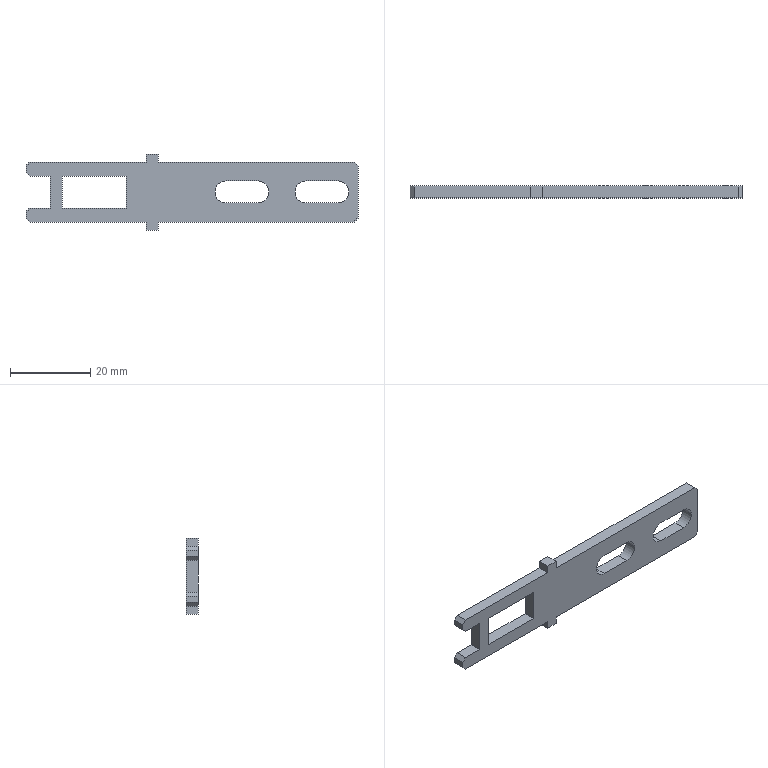Part | NX | features solid 2 | 1 solid | 38 faces | box 83 x 3 x 19 mm | volume 2827 mm3 | plane 32 | cylinder 6 | commonest cylinder face diameters 5.5 x6
STEP:
#1=CARTESIAN_POINT('',(-284.034,-1543.5,1313.749));
#2=VERTEX_POINT('',#1);
#3=CARTESIAN_POINT('',(-284.034,-1540.5,1313.749));
#4=VERTEX_POINT('',#3);
#5=CARTESIAN_POINT('',(-284.034,-1625.7,1313.749));
#6=DIRECTION('',(0.,1.,0.));
#7=VECTOR('',#6,1000.);
#8=LINE('',#5,#7);
#9=EDGE_CURVE('',#2,#4,#8,.T.);
#10=ORIENTED_EDGE('',*,*,#9,.T.);
#11=CARTESIAN_POINT('',(-276.034,-1540.5,1313.749));
#12=VERTEX_POINT('',#11);
#13=CARTESIAN_POINT('',(-284.034,-1540.5,1313.749));
#14=DIRECTION('',(1.,0.,0.));
#15=VECTOR('',#14,1000.);
#16=LINE('',#13,#15);
#17=EDGE_CURVE('',#4,#12,#16,.T.);
#18=ORIENTED_EDGE('',*,*,#17,.T.);
#19=CARTESIAN_POINT('',(-276.034,-1543.5,1313.749));
#20=VERTEX_POINT('',#19);
#21=CARTESIAN_POINT('',(-276.034,-1625.7,1313.749));
#22=DIRECTION('',(0.,1.,0.));
#23=VECTOR('',#22,1000.);
#24=LINE('',#21,#23);
#25=EDGE_CURVE('',#20,#12,#24,.T.);
#26=ORIENTED_EDGE('',*,*,#25,.F.);
#27=CARTESIAN_POINT('',(-354.034,-1543.5,1313.749));
#28=DIRECTION('',(1.,0.,0.));
#29=VECTOR('',#28,1000.);
#30=LINE('',#27,#29);
#31=EDGE_CURVE('',#2,#20,#30,.T.);
#32=ORIENTED_EDGE('',*,*,#31,.F.);
#33=EDGE_LOOP('',(#10,#18,#26,#32));
#34=FACE_BOUND('',#33,.T.);
#35=CARTESIAN_POINT('',(-284.034,-1625.7,1313.749));
#36=DIRECTION('',(0.,0.,1.));
#37=DIRECTION('',(1.,0.,0.));
#38=AXIS2_PLACEMENT_3D('',#35,#36,#37);
#39=PLANE('',#38);
#40=ADVANCED_FACE('',(#34),#39,.F.);
#41=CARTESIAN_POINT('',(-284.034,-1543.5,1308.249));
#42=VERTEX_POINT('',#41);
#43=CARTESIAN_POINT('',(-284.034,-1540.5,1308.249));
#44=VERTEX_POINT('',#43);
#45=CARTESIAN_POINT('',(-284.034,-1625.7,1308.249));
#46=DIRECTION('',(0.,1.,0.));
#47=VECTOR('',#46,1000.);
#48=LINE('',#45,#47);
#49=EDGE_CURVE('',#42,#44,#48,.T.);
#50=ORIENTED_EDGE('',*,*,#49,.T.);
#51=CARTESIAN_POINT('',(-284.034,-1540.5,1310.999));
#52=DIRECTION('',(0.,1.,0.));
#53=DIRECTION('',(1.,0.,0.));
#54=AXIS2_PLACEMENT_3D('',#51,#52,#53);
#55=CIRCLE('',#54,2.75);
#56=EDGE_CURVE('',#44,#4,#55,.T.);
#57=ORIENTED_EDGE('',*,*,#56,.T.);
#58=ORIENTED_EDGE('',*,*,#9,.F.);
#59=CARTESIAN_POINT('',(-284.034,-1543.5,1310.999));
#60=DIRECTION('',(0.,1.,0.));
#61=DIRECTION('',(1.,0.,0.));
#62=AXIS2_PLACEMENT_3D('',#59,#60,#61);
#63=CIRCLE('',#62,2.75);
#64=EDGE_CURVE('',#42,#2,#63,.T.);
#65=ORIENTED_EDGE('',*,*,#64,.F.);
#66=EDGE_LOOP('',(#50,#57,#58,#65));
#67=FACE_BOUND('',#66,.T.);
#68=CARTESIAN_POINT('',(-284.034,-1625.7,1310.999));
#69=DIRECTION('',(0.,1.,0.));
#70=DIRECTION('',(1.,0.,0.));
#71=AXIS2_PLACEMENT_3D('',#68,#69,#70);
#72=CYLINDRICAL_SURFACE('',#71,2.75);
#73=ADVANCED_FACE('',(#67),#72,.F.);
#74=CARTESIAN_POINT('',(-276.034,-1543.5,1308.249));
#75=VERTEX_POINT('',#74);
#76=CARTESIAN_POINT('',(-276.034,-1540.5,1308.249));
#77=VERTEX_POINT('',#76);
#78=CARTESIAN_POINT('',(-276.034,-1625.7,1308.249));
#79=DIRECTION('',(0.,1.,0.));
#80=VECTOR('',#79,1000.);
#81=LINE('',#78,#80);
#82=EDGE_CURVE('',#75,#77,#81,.T.);
#83=ORIENTED_EDGE('',*,*,#82,.T.);
#84=CARTESIAN_POINT('',(-284.034,-1540.5,1308.249));
#85=DIRECTION('',(-1.,0.,0.));
#86=VECTOR('',#85,1000.);
#87=LINE('',#84,#86);
#88=EDGE_CURVE('',#77,#44,#87,.T.);
#89=ORIENTED_EDGE('',*,*,#88,.T.);
#90=ORIENTED_EDGE('',*,*,#49,.F.);
#91=CARTESIAN_POINT('',(-354.034,-1543.5,1308.249));
#92=DIRECTION('',(-1.,0.,0.));
#93=VECTOR('',#92,1000.);
#94=LINE('',#91,#93);
#95=EDGE_CURVE('',#75,#42,#94,.T.);
#96=ORIENTED_EDGE('',*,*,#95,.F.);
#97=EDGE_LOOP('',(#83,#89,#90,#96));
#98=FACE_BOUND('',#97,.T.);
#99=CARTESIAN_POINT('',(-284.034,-1625.7,1308.249));
#100=DIRECTION('',(0.,0.,-1.));
#101=DIRECTION('',(-1.,0.,0.));
#102=AXIS2_PLACEMENT_3D('',#99,#100,#101);
#103=PLANE('',#102);
#104=ADVANCED_FACE('',(#98),#103,.F.);
#105=CARTESIAN_POINT('',(-273.284,-1543.5,1310.999));
#106=VERTEX_POINT('',#105);
#107=CARTESIAN_POINT('',(-273.284,-1540.5,1310.999));
#108=VERTEX_POINT('',#107);
#109=CARTESIAN_POINT('',(-273.284,-1625.7,1310.999));
#110=DIRECTION('',(0.,1.,0.));
#111=VECTOR('',#110,1000.);
#112=LINE('',#109,#111);
#113=EDGE_CURVE('',#106,#108,#112,.T.);
#114=ORIENTED_EDGE('',*,*,#113,.F.);
#115=CARTESIAN_POINT('',(-276.034,-1543.5,1310.999));
#116=DIRECTION('',(0.,1.,0.));
#117=DIRECTION('',(1.,0.,0.));
#118=AXIS2_PLACEMENT_3D('',#115,#116,#117);
#119=CIRCLE('',#118,2.75);
#120=EDGE_CURVE('',#20,#106,#119,.T.);
#121=ORIENTED_EDGE('',*,*,#120,.F.);
#122=ORIENTED_EDGE('',*,*,#25,.T.);
#123=CARTESIAN_POINT('',(-276.034,-1540.5,1310.999));
#124=DIRECTION('',(0.,1.,0.));
#125=DIRECTION('',(-1.,0.,0.));
#126=AXIS2_PLACEMENT_3D('',#123,#124,#125);
#127=CIRCLE('',#126,2.75);
#128=EDGE_CURVE('',#12,#108,#127,.T.);
#129=ORIENTED_EDGE('',*,*,#128,.T.);
#130=EDGE_LOOP('',(#114,#121,#122,#129));
#131=FACE_BOUND('',#130,.T.);
#132=CARTESIAN_POINT('',(-276.034,-1625.7,1310.999));
#133=DIRECTION('',(0.,1.,0.));
#134=DIRECTION('',(1.,0.,0.));
#135=AXIS2_PLACEMENT_3D('',#132,#133,#134);
#136=CYLINDRICAL_SURFACE('',#135,2.75);
#137=ADVANCED_FACE('',(#131),#136,.F.);
#138=CARTESIAN_POINT('',(-304.034,-1543.5,1313.749));
#139=VERTEX_POINT('',#138);
#140=CARTESIAN_POINT('',(-304.034,-1540.5,1313.749));
#141=VERTEX_POINT('',#140);
#142=CARTESIAN_POINT('',(-304.034,-1625.7,1313.749));
#143=DIRECTION('',(0.,1.,0.));
#144=VECTOR('',#143,1000.);
#145=LINE('',#142,#144);
#146=EDGE_CURVE('',#139,#141,#145,.T.);
#147=ORIENTED_EDGE('',*,*,#146,.T.);
#148=CARTESIAN_POINT('',(-296.034,-1540.5,1313.749));
#149=VERTEX_POINT('',#148);
#150=CARTESIAN_POINT('',(-304.034,-1540.5,1313.749));
#151=DIRECTION('',(1.,0.,0.));
#152=VECTOR('',#151,1000.);
#153=LINE('',#150,#152);
#154=EDGE_CURVE('',#141,#149,#153,.T.);
#155=ORIENTED_EDGE('',*,*,#154,.T.);
#156=CARTESIAN_POINT('',(-296.034,-1543.5,1313.749));
#157=VERTEX_POINT('',#156);
#158=CARTESIAN_POINT('',(-296.034,-1625.7,1313.749));
#159=DIRECTION('',(0.,1.,0.));
#160=VECTOR('',#159,1000.);
#161=LINE('',#158,#160);
#162=EDGE_CURVE('',#157,#149,#161,.T.);
#163=ORIENTED_EDGE('',*,*,#162,.F.);
#164=CARTESIAN_POINT('',(-354.034,-1543.5,1313.749));
#165=DIRECTION('',(1.,0.,0.));
#166=VECTOR('',#165,1000.);
#167=LINE('',#164,#166);
#168=EDGE_CURVE('',#139,#157,#167,.T.);
#169=ORIENTED_EDGE('',*,*,#168,.F.);
#170=EDGE_LOOP('',(#147,#155,#163,#169));
#171=FACE_BOUND('',#170,.T.);
#172=CARTESIAN_POINT('',(-304.034,-1625.7,1313.749));
#173=DIRECTION('',(0.,0.,1.));
#174=DIRECTION('',(1.,0.,0.));
#175=AXIS2_PLACEMENT_3D('',#172,#173,#174);
#176=PLANE('',#175);
#177=ADVANCED_FACE('',(#171),#176,.F.);
#178=CARTESIAN_POINT('',(-304.034,-1543.5,1308.249));
#179=VERTEX_POINT('',#178);
#180=CARTESIAN_POINT('',(-304.034,-1540.5,1308.249));
#181=VERTEX_POINT('',#180);
#182=CARTESIAN_POINT('',(-304.034,-1625.7,1308.249));
#183=DIRECTION('',(0.,1.,0.));
#184=VECTOR('',#183,1000.);
#185=LINE('',#182,#184);
#186=EDGE_CURVE('',#179,#181,#185,.T.);
#187=ORIENTED_EDGE('',*,*,#186,.T.);
#188=CARTESIAN_POINT('',(-304.034,-1540.5,1310.999));
#189=DIRECTION('',(0.,1.,0.));
#190=DIRECTION('',(1.,0.,0.));
#191=AXIS2_PLACEMENT_3D('',#188,#189,#190);
#192=CIRCLE('',#191,2.75);
#193=EDGE_CURVE('',#181,#141,#192,.T.);
#194=ORIENTED_EDGE('',*,*,#193,.T.);
#195=ORIENTED_EDGE('',*,*,#146,.F.);
#196=CARTESIAN_POINT('',(-304.034,-1543.5,1310.999));
#197=DIRECTION('',(0.,1.,0.));
#198=DIRECTION('',(1.,0.,0.));
#199=AXIS2_PLACEMENT_3D('',#196,#197,#198);
#200=CIRCLE('',#199,2.75);
#201=EDGE_CURVE('',#179,#139,#200,.T.);
#202=ORIENTED_EDGE('',*,*,#201,.F.);
#203=EDGE_LOOP('',(#187,#194,#195,#202));
#204=FACE_BOUND('',#203,.T.);
#205=CARTESIAN_POINT('',(-304.034,-1625.7,1310.999));
#206=DIRECTION('',(0.,1.,0.));
#207=DIRECTION('',(1.,0.,0.));
#208=AXIS2_PLACEMENT_3D('',#205,#206,#207);
#209=CYLINDRICAL_SURFACE('',#208,2.75);
#210=ADVANCED_FACE('',(#204),#209,.F.);
#211=CARTESIAN_POINT('',(-296.034,-1543.5,1308.249));
#212=VERTEX_POINT('',#211);
#213=CARTESIAN_POINT('',(-296.034,-1540.5,1308.249));
#214=VERTEX_POINT('',#213);
#215=CARTESIAN_POINT('',(-296.034,-1625.7,1308.249));
#216=DIRECTION('',(0.,1.,0.));
#217=VECTOR('',#216,1000.);
#218=LINE('',#215,#217);
#219=EDGE_CURVE('',#212,#214,#218,.T.);
#220=ORIENTED_EDGE('',*,*,#219,.T.);
#221=CARTESIAN_POINT('',(-304.034,-1540.5,1308.249));
#222=DIRECTION('',(-1.,0.,0.));
#223=VECTOR('',#222,1000.);
#224=LINE('',#221,#223);
#225=EDGE_CURVE('',#214,#181,#224,.T.);
#226=ORIENTED_EDGE('',*,*,#225,.T.);
#227=ORIENTED_EDGE('',*,*,#186,.F.);
#228=CARTESIAN_POINT('',(-354.034,-1543.5,1308.249));
#229=DIRECTION('',(-1.,0.,0.));
#230=VECTOR('',#229,1000.);
#231=LINE('',#228,#230);
#232=EDGE_CURVE('',#212,#179,#231,.T.);
#233=ORIENTED_EDGE('',*,*,#232,.F.);
#234=EDGE_LOOP('',(#220,#226,#227,#233));
#235=FACE_BOUND('',#234,.T.);
#236=CARTESIAN_POINT('',(-304.034,-1625.7,1308.249));
#237=DIRECTION('',(0.,0.,-1.));
#238=DIRECTION('',(-1.,0.,0.));
#239=AXIS2_PLACEMENT_3D('',#236,#237,#238);
#240=PLANE('',#239);
#241=ADVANCED_FACE('',(#235),#240,.F.);
#242=CARTESIAN_POINT('',(-293.284,-1543.5,1310.999));
#243=VERTEX_POINT('',#242);
#244=CARTESIAN_POINT('',(-293.284,-1540.5,1310.999));
#245=VERTEX_POINT('',#244);
#246=CARTESIAN_POINT('',(-293.284,-1625.7,1310.999));
#247=DIRECTION('',(0.,1.,0.));
#248=VECTOR('',#247,1000.);
#249=LINE('',#246,#248);
#250=EDGE_CURVE('',#243,#245,#249,.T.);
#251=ORIENTED_EDGE('',*,*,#250,.F.);
#252=CARTESIAN_POINT('',(-296.034,-1543.5,1310.999));
#253=DIRECTION('',(0.,1.,0.));
#254=DIRECTION('',(1.,0.,0.));
#255=AXIS2_PLACEMENT_3D('',#252,#253,#254);
#256=CIRCLE('',#255,2.75);
#257=EDGE_CURVE('',#157,#243,#256,.T.);
#258=ORIENTED_EDGE('',*,*,#257,.F.);
#259=ORIENTED_EDGE('',*,*,#162,.T.);
#260=CARTESIAN_POINT('',(-296.034,-1540.5,1310.999));
#261=DIRECTION('',(0.,1.,0.));
#262=DIRECTION('',(-1.,0.,0.));
#263=AXIS2_PLACEMENT_3D('',#260,#261,#262);
#264=CIRCLE('',#263,2.75);
#265=EDGE_CURVE('',#149,#245,#264,.T.);
#266=ORIENTED_EDGE('',*,*,#265,.T.);
#267=EDGE_LOOP('',(#251,#258,#259,#266));
#268=FACE_BOUND('',#267,.T.);
#269=CARTESIAN_POINT('',(-296.034,-1625.7,1310.999));
#270=DIRECTION('',(0.,1.,0.));
#271=DIRECTION('',(1.,0.,0.));
#272=AXIS2_PLACEMENT_3D('',#269,#270,#271);
#273=CYLINDRICAL_SURFACE('',#272,2.75);
#274=ADVANCED_FACE('',(#268),#273,.F.);
#275=CARTESIAN_POINT('',(-354.034,-1543.5,1304.499));
#276=VERTEX_POINT('',#275);
#277=CARTESIAN_POINT('',(-353.034,-1543.5,1303.499));
#278=VERTEX_POINT('',#277);
#279=CARTESIAN_POINT('',(-353.034,-1543.5,1303.499));
#280=DIRECTION('',(0.7071,0.,-0.7071));
#281=VECTOR('',#280,1000.);
#282=LINE('',#279,#281);
#283=EDGE_CURVE('',#276,#278,#282,.T.);
#284=ORIENTED_EDGE('',*,*,#283,.F.);
#285=CARTESIAN_POINT('',(-354.034,-1540.5,1304.499));
#286=VERTEX_POINT('',#285);
#287=CARTESIAN_POINT('',(-354.034,-1543.5,1304.499));
#288=DIRECTION('',(0.,-1.,0.));
#289=VECTOR('',#288,1000.);
#290=LINE('',#287,#289);
#291=EDGE_CURVE('',#286,#276,#290,.T.);
#292=ORIENTED_EDGE('',*,*,#291,.F.);
#293=CARTESIAN_POINT('',(-353.034,-1540.5,1303.499));
#294=VERTEX_POINT('',#293);
#295=CARTESIAN_POINT('',(-362.034,-1540.5,1312.499));
#296=DIRECTION('',(-0.7071,0.,0.7071));
#297=VECTOR('',#296,1000.);
#298=LINE('',#295,#297);
#299=EDGE_CURVE('',#294,#286,#298,.T.);
#300=ORIENTED_EDGE('',*,*,#299,.F.);
#301=CARTESIAN_POINT('',(-353.034,-1540.5,1303.499));
#302=DIRECTION('',(0.,1.,0.));
#303=VECTOR('',#302,1000.);
#304=LINE('',#301,#303);
#305=EDGE_CURVE('',#278,#294,#304,.T.);
#306=ORIENTED_EDGE('',*,*,#305,.F.);
#307=EDGE_LOOP('',(#284,#292,#300,#306));
#308=FACE_BOUND('',#307,.T.);
#309=CARTESIAN_POINT('',(-353.034,-1540.5,1303.499));
#310=DIRECTION('',(-0.7071,0.,-0.7071));
#311=DIRECTION('',(-0.7071,0.,0.7071));
#312=AXIS2_PLACEMENT_3D('',#309,#310,#311);
#313=PLANE('',#312);
#314=ADVANCED_FACE('',(#308),#313,.T.);
#315=CARTESIAN_POINT('',(-353.034,-1543.5,1306.999));
#316=VERTEX_POINT('',#315);
#317=CARTESIAN_POINT('',(-354.034,-1543.5,1305.999));
#318=VERTEX_POINT('',#317);
#319=CARTESIAN_POINT('',(-354.034,-1543.5,1305.999));
#320=DIRECTION('',(-0.7071,0.,-0.7071));
#321=VECTOR('',#320,1000.);
#322=LINE('',#319,#321);
#323=EDGE_CURVE('',#316,#318,#322,.T.);
#324=ORIENTED_EDGE('',*,*,#323,.F.);
#325=CARTESIAN_POINT('',(-353.034,-1540.5,1306.999));
#326=VERTEX_POINT('',#325);
#327=CARTESIAN_POINT('',(-353.034,-1543.5,1306.999));
#328=DIRECTION('',(0.,-1.,0.));
#329=VECTOR('',#328,1000.);
#330=LINE('',#327,#329);
#331=EDGE_CURVE('',#326,#316,#330,.T.);
#332=ORIENTED_EDGE('',*,*,#331,.F.);
#333=CARTESIAN_POINT('',(-354.034,-1540.5,1305.999));
#334=VERTEX_POINT('',#333);
#335=CARTESIAN_POINT('',(-346.784,-1540.5,1313.249));
#336=DIRECTION('',(0.7071,0.,0.7071));
#337=VECTOR('',#336,1000.);
#338=LINE('',#335,#337);
#339=EDGE_CURVE('',#334,#326,#338,.T.);
#340=ORIENTED_EDGE('',*,*,#339,.F.);
#341=CARTESIAN_POINT('',(-354.034,-1540.5,1305.999));
#342=DIRECTION('',(0.,1.,0.));
#343=VECTOR('',#342,1000.);
#344=LINE('',#341,#343);
#345=EDGE_CURVE('',#318,#334,#344,.T.);
#346=ORIENTED_EDGE('',*,*,#345,.F.);
#347=EDGE_LOOP('',(#324,#332,#340,#346));
#348=FACE_BOUND('',#347,.T.);
#349=CARTESIAN_POINT('',(-354.034,-1543.5,1305.999));
#350=DIRECTION('',(-0.7071,0.,0.7071));
#351=DIRECTION('',(0.,1.,0.));
#352=AXIS2_PLACEMENT_3D('',#349,#350,#351);
#353=PLANE('',#352);
#354=ADVANCED_FACE('',(#348),#353,.T.);
#355=CARTESIAN_POINT('',(-354.034,-1543.5,1315.999));
#356=VERTEX_POINT('',#355);
#357=CARTESIAN_POINT('',(-353.034,-1543.5,1314.999));
#358=VERTEX_POINT('',#357);
#359=CARTESIAN_POINT('',(-353.034,-1543.5,1314.999));
#360=DIRECTION('',(0.7071,0.,-0.7071));
#361=VECTOR('',#360,1000.);
#362=LINE('',#359,#361);
#363=EDGE_CURVE('',#356,#358,#362,.T.);
#364=ORIENTED_EDGE('',*,*,#363,.F.);
#365=CARTESIAN_POINT('',(-354.034,-1540.5,1315.999));
#366=VERTEX_POINT('',#365);
#367=CARTESIAN_POINT('',(-354.034,-1543.5,1315.999));
#368=DIRECTION('',(0.,-1.,0.));
#369=VECTOR('',#368,1000.);
#370=LINE('',#367,#369);
#371=EDGE_CURVE('',#366,#356,#370,.T.);
#372=ORIENTED_EDGE('',*,*,#371,.F.);
#373=CARTESIAN_POINT('',(-353.034,-1540.5,1314.999));
#374=VERTEX_POINT('',#373);
#375=CARTESIAN_POINT('',(-356.284,-1540.5,1318.249));
#376=DIRECTION('',(-0.7071,0.,0.7071));
#377=VECTOR('',#376,1000.);
#378=LINE('',#375,#377);
#379=EDGE_CURVE('',#374,#366,#378,.T.);
#380=ORIENTED_EDGE('',*,*,#379,.F.);
#381=CARTESIAN_POINT('',(-353.034,-1540.5,1314.999));
#382=DIRECTION('',(0.,1.,0.));
#383=VECTOR('',#382,1000.);
#384=LINE('',#381,#383);
#385=EDGE_CURVE('',#358,#374,#384,.T.);
#386=ORIENTED_EDGE('',*,*,#385,.F.);
#387=EDGE_LOOP('',(#364,#372,#380,#386));
#388=FACE_BOUND('',#387,.T.);
#389=CARTESIAN_POINT('',(-353.034,-1540.5,1314.999));
#390=DIRECTION('',(-0.7071,0.,-0.7071));
#391=DIRECTION('',(-0.7071,0.,0.7071));
#392=AXIS2_PLACEMENT_3D('',#389,#390,#391);
#393=PLANE('',#392);
#394=ADVANCED_FACE('',(#388),#393,.T.);
#395=CARTESIAN_POINT('',(-353.034,-1543.5,1318.499));
#396=VERTEX_POINT('',#395);
#397=CARTESIAN_POINT('',(-354.034,-1543.5,1317.499));
#398=VERTEX_POINT('',#397);
#399=CARTESIAN_POINT('',(-354.034,-1543.5,1317.499));
#400=DIRECTION('',(-0.7071,0.,-0.7071));
#401=VECTOR('',#400,1000.);
#402=LINE('',#399,#401);
#403=EDGE_CURVE('',#396,#398,#402,.T.);
#404=ORIENTED_EDGE('',*,*,#403,.F.);
#405=CARTESIAN_POINT('',(-353.034,-1540.5,1318.499));
#406=VERTEX_POINT('',#405);
#407=CARTESIAN_POINT('',(-353.034,-1543.5,1318.499));
#408=DIRECTION('',(0.,-1.,0.));
#409=VECTOR('',#408,1000.);
#410=LINE('',#407,#409);
#411=EDGE_CURVE('',#406,#396,#410,.T.);
#412=ORIENTED_EDGE('',*,*,#411,.F.);
#413=CARTESIAN_POINT('',(-354.034,-1540.5,1317.499));
#414=VERTEX_POINT('',#413);
#415=CARTESIAN_POINT('',(-352.534,-1540.5,1318.999));
#416=DIRECTION('',(0.7071,0.,0.7071));
#417=VECTOR('',#416,1000.);
#418=LINE('',#415,#417);
#419=EDGE_CURVE('',#414,#406,#418,.T.);
#420=ORIENTED_EDGE('',*,*,#419,.F.);
#421=CARTESIAN_POINT('',(-354.034,-1540.5,1317.499));
#422=DIRECTION('',(0.,1.,0.));
#423=VECTOR('',#422,1000.);
#424=LINE('',#421,#423);
#425=EDGE_CURVE('',#398,#414,#424,.T.);
#426=ORIENTED_EDGE('',*,*,#425,.F.);
#427=EDGE_LOOP('',(#404,#412,#420,#426));
#428=FACE_BOUND('',#427,.T.);
#429=CARTESIAN_POINT('',(-354.034,-1543.5,1317.499));
#430=DIRECTION('',(0.7071,0.,-0.7071));
#431=DIRECTION('',(0.,-1.,0.));
#432=AXIS2_PLACEMENT_3D('',#429,#430,#431);
#433=PLANE('',#432);
#434=ADVANCED_FACE('',(#428),#433,.F.);
#435=CARTESIAN_POINT('',(-272.034,-1543.5,1303.499));
#436=VERTEX_POINT('',#435);
#437=CARTESIAN_POINT('',(-271.034,-1543.5,1304.499));
#438=VERTEX_POINT('',#437);
#439=CARTESIAN_POINT('',(-271.034,-1543.5,1304.499));
#440=DIRECTION('',(0.7071,0.,0.7071));
#441=VECTOR('',#440,1000.);
#442=LINE('',#439,#441);
#443=EDGE_CURVE('',#436,#438,#442,.T.);
#444=ORIENTED_EDGE('',*,*,#443,.F.);
#445=CARTESIAN_POINT('',(-272.034,-1540.5,1303.499));
#446=VERTEX_POINT('',#445);
#447=CARTESIAN_POINT('',(-272.034,-1543.5,1303.499));
#448=DIRECTION('',(0.,-1.,0.));
#449=VECTOR('',#448,1000.);
#450=LINE('',#447,#449);
#451=EDGE_CURVE('',#446,#436,#450,.T.);
#452=ORIENTED_EDGE('',*,*,#451,.F.);
#453=CARTESIAN_POINT('',(-271.034,-1540.5,1304.499));
#454=VERTEX_POINT('',#453);
#455=CARTESIAN_POINT('',(-304.534,-1540.5,1270.999));
#456=DIRECTION('',(-0.7071,0.,-0.7071));
#457=VECTOR('',#456,1000.);
#458=LINE('',#455,#457);
#459=EDGE_CURVE('',#454,#446,#458,.T.);
#460=ORIENTED_EDGE('',*,*,#459,.F.);
#461=CARTESIAN_POINT('',(-271.034,-1540.5,1304.499));
#462=DIRECTION('',(0.,1.,0.));
#463=VECTOR('',#462,1000.);
#464=LINE('',#461,#463);
#465=EDGE_CURVE('',#438,#454,#464,.T.);
#466=ORIENTED_EDGE('',*,*,#465,.F.);
#467=EDGE_LOOP('',(#444,#452,#460,#466));
#468=FACE_BOUND('',#467,.T.);
#469=CARTESIAN_POINT('',(-271.034,-1543.5,1304.499));
#470=DIRECTION('',(0.7071,0.,-0.7071));
#471=DIRECTION('',(0.,-1.,0.));
#472=AXIS2_PLACEMENT_3D('',#469,#470,#471);
#473=PLANE('',#472);
#474=ADVANCED_FACE('',(#468),#473,.T.);
#475=CARTESIAN_POINT('',(-271.034,-1543.5,1317.499));
#476=VERTEX_POINT('',#475);
#477=CARTESIAN_POINT('',(-272.034,-1543.5,1318.499));
#478=VERTEX_POINT('',#477);
#479=CARTESIAN_POINT('',(-272.034,-1543.5,1318.499));
#480=DIRECTION('',(-0.7071,0.,0.7071));
#481=VECTOR('',#480,1000.);
#482=LINE('',#479,#481);
#483=EDGE_CURVE('',#476,#478,#482,.T.);
#484=ORIENTED_EDGE('',*,*,#483,.F.);
#485=CARTESIAN_POINT('',(-271.034,-1540.5,1317.499));
#486=VERTEX_POINT('',#485);
#487=CARTESIAN_POINT('',(-271.034,-1543.5,1317.499));
#488=DIRECTION('',(0.,-1.,0.));
#489=VECTOR('',#488,1000.);
#490=LINE('',#487,#489);
#491=EDGE_CURVE('',#486,#476,#490,.T.);
#492=ORIENTED_EDGE('',*,*,#491,.F.);
#493=CARTESIAN_POINT('',(-272.034,-1540.5,1318.499));
#494=VERTEX_POINT('',#493);
#495=CARTESIAN_POINT('',(-314.034,-1540.5,1360.499));
#496=DIRECTION('',(0.7071,0.,-0.7071));
#497=VECTOR('',#496,1000.);
#498=LINE('',#495,#497);
#499=EDGE_CURVE('',#494,#486,#498,.T.);
#500=ORIENTED_EDGE('',*,*,#499,.F.);
#501=CARTESIAN_POINT('',(-272.034,-1540.5,1318.499));
#502=DIRECTION('',(0.,1.,0.));
#503=VECTOR('',#502,1000.);
#504=LINE('',#501,#503);
#505=EDGE_CURVE('',#478,#494,#504,.T.);
#506=ORIENTED_EDGE('',*,*,#505,.F.);
#507=EDGE_LOOP('',(#484,#492,#500,#506));
#508=FACE_BOUND('',#507,.T.);
#509=CARTESIAN_POINT('',(-272.034,-1540.5,1318.499));
#510=DIRECTION('',(-0.7071,0.,-0.7071));
#511=DIRECTION('',(-0.7071,0.,0.7071));
#512=AXIS2_PLACEMENT_3D('',#509,#510,#511);
#513=PLANE('',#512);
#514=ADVANCED_FACE('',(#508),#513,.F.);
#515=CARTESIAN_POINT('',(-348.034,-1540.5,1306.999));
#516=VERTEX_POINT('',#515);
#517=CARTESIAN_POINT('',(-354.034,-1540.5,1306.999));
#518=DIRECTION('',(-1.,0.,0.));
#519=VECTOR('',#518,1000.);
#520=LINE('',#517,#519);
#521=EDGE_CURVE('',#516,#326,#520,.T.);
#522=ORIENTED_EDGE('',*,*,#521,.T.);
#523=ORIENTED_EDGE('',*,*,#331,.T.);
#524=CARTESIAN_POINT('',(-348.034,-1543.5,1306.999));
#525=VERTEX_POINT('',#524);
#526=CARTESIAN_POINT('',(-354.034,-1543.5,1306.999));
#527=DIRECTION('',(-1.,0.,0.));
#528=VECTOR('',#527,1000.);
#529=LINE('',#526,#528);
#530=EDGE_CURVE('',#525,#316,#529,.T.);
#531=ORIENTED_EDGE('',*,*,#530,.F.);
#532=CARTESIAN_POINT('',(-348.034,-1540.5,1306.999));
#533=DIRECTION('',(0.,1.,0.));
#534=VECTOR('',#533,1000.);
#535=LINE('',#532,#534);
#536=EDGE_CURVE('',#525,#516,#535,.T.);
#537=ORIENTED_EDGE('',*,*,#536,.T.);
#538=EDGE_LOOP('',(#522,#523,#531,#537));
#539=FACE_BOUND('',#538,.T.);
#540=CARTESIAN_POINT('',(-354.034,-1540.5,1306.999));
#541=DIRECTION('',(0.,0.,-1.));
#542=DIRECTION('',(0.,-1.,0.));
#543=AXIS2_PLACEMENT_3D('',#540,#541,#542);
#544=PLANE('',#543);
#545=ADVANCED_FACE('',(#539),#544,.F.);
#546=CARTESIAN_POINT('',(-348.034,-1543.5,1314.999));
#547=VERTEX_POINT('',#546);
#548=CARTESIAN_POINT('',(-348.034,-1540.5,1314.999));
#549=VERTEX_POINT('',#548);
#550=CARTESIAN_POINT('',(-348.034,-1540.5,1314.999));
#551=DIRECTION('',(0.,1.,0.));
#552=VECTOR('',#551,1000.);
#553=LINE('',#550,#552);
#554=EDGE_CURVE('',#547,#549,#553,.T.);
#555=ORIENTED_EDGE('',*,*,#554,.T.);
#556=CARTESIAN_POINT('',(-348.034,-1540.5,1320.499));
#557=DIRECTION('',(0.,0.,-1.));
#558=VECTOR('',#557,1000.);
#559=LINE('',#556,#558);
#560=EDGE_CURVE('',#549,#516,#559,.T.);
#561=ORIENTED_EDGE('',*,*,#560,.T.);
#562=ORIENTED_EDGE('',*,*,#536,.F.);
#563=CARTESIAN_POINT('',(-348.034,-1543.5,1320.499));
#564=DIRECTION('',(0.,0.,-1.));
#565=VECTOR('',#564,1000.);
#566=LINE('',#563,#565);
#567=EDGE_CURVE('',#547,#525,#566,.T.);
#568=ORIENTED_EDGE('',*,*,#567,.F.);
#569=EDGE_LOOP('',(#555,#561,#562,#568));
#570=FACE_BOUND('',#569,.T.);
#571=CARTESIAN_POINT('',(-348.034,-1540.5,1320.499));
#572=DIRECTION('',(1.,0.,0.));
#573=DIRECTION('',(0.,1.,0.));
#574=AXIS2_PLACEMENT_3D('',#571,#572,#573);
#575=PLANE('',#574);
#576=ADVANCED_FACE('',(#570),#575,.F.);
#577=CARTESIAN_POINT('',(-354.034,-1543.5,1314.999));
#578=DIRECTION('',(1.,0.,0.));
#579=VECTOR('',#578,1000.);
#580=LINE('',#577,#579);
#581=EDGE_CURVE('',#358,#547,#580,.T.);
#582=ORIENTED_EDGE('',*,*,#581,.F.);
#583=ORIENTED_EDGE('',*,*,#385,.T.);
#584=CARTESIAN_POINT('',(-354.034,-1540.5,1314.999));
#585=DIRECTION('',(1.,0.,0.));
#586=VECTOR('',#585,1000.);
#587=LINE('',#584,#586);
#588=EDGE_CURVE('',#374,#549,#587,.T.);
#589=ORIENTED_EDGE('',*,*,#588,.T.);
#590=ORIENTED_EDGE('',*,*,#554,.F.);
#591=EDGE_LOOP('',(#582,#583,#589,#590));
#592=FACE_BOUND('',#591,.T.);
#593=CARTESIAN_POINT('',(-354.034,-1540.5,1314.999));
#594=DIRECTION('',(0.,0.,1.));
#595=DIRECTION('',(0.,-1.,0.));
#596=AXIS2_PLACEMENT_3D('',#593,#594,#595);
#597=PLANE('',#596);
#598=ADVANCED_FACE('',(#592),#597,.F.);
#599=CARTESIAN_POINT('',(-345.034,-1543.5,1314.999));
#600=VERTEX_POINT('',#599);
#601=CARTESIAN_POINT('',(-345.034,-1540.5,1314.999));
#602=VERTEX_POINT('',#601);
#603=CARTESIAN_POINT('',(-345.034,-1625.7,1314.999));
#604=DIRECTION('',(0.,1.,0.));
#605=VECTOR('',#604,1000.);
#606=LINE('',#603,#605);
#607=EDGE_CURVE('',#600,#602,#606,.T.);
#608=ORIENTED_EDGE('',*,*,#607,.T.);
#609=CARTESIAN_POINT('',(-329.034,-1540.5,1314.999));
#610=VERTEX_POINT('',#609);
#611=CARTESIAN_POINT('',(-345.034,-1540.5,1314.999));
#612=DIRECTION('',(1.,0.,0.));
#613=VECTOR('',#612,1000.);
#614=LINE('',#611,#613);
#615=EDGE_CURVE('',#602,#610,#614,.T.);
#616=ORIENTED_EDGE('',*,*,#615,.T.);
#617=CARTESIAN_POINT('',(-329.034,-1543.5,1314.999));
#618=VERTEX_POINT('',#617);
#619=CARTESIAN_POINT('',(-329.034,-1625.7,1314.999));
#620=DIRECTION('',(0.,1.,0.));
#621=VECTOR('',#620,1000.);
#622=LINE('',#619,#621);
#623=EDGE_CURVE('',#618,#610,#622,.T.);
#624=ORIENTED_EDGE('',*,*,#623,.F.);
#625=CARTESIAN_POINT('',(-354.034,-1543.5,1314.999));
#626=DIRECTION('',(1.,0.,0.));
#627=VECTOR('',#626,1000.);
#628=LINE('',#625,#627);
#629=EDGE_CURVE('',#600,#618,#628,.T.);
#630=ORIENTED_EDGE('',*,*,#629,.F.);
#631=EDGE_LOOP('',(#608,#616,#624,#630));
#632=FACE_BOUND('',#631,.T.);
#633=CARTESIAN_POINT('',(-345.034,-1625.7,1314.999));
#634=DIRECTION('',(0.,0.,1.));
#635=DIRECTION('',(1.,0.,0.));
#636=AXIS2_PLACEMENT_3D('',#633,#634,#635);
#637=PLANE('',#636);
#638=ADVANCED_FACE('',(#632),#637,.F.);
#639=CARTESIAN_POINT('',(-345.034,-1543.5,1306.999));
#640=VERTEX_POINT('',#639);
#641=CARTESIAN_POINT('',(-345.034,-1540.5,1306.999));
#642=VERTEX_POINT('',#641);
#643=CARTESIAN_POINT('',(-345.034,-1625.7,1306.999));
#644=DIRECTION('',(0.,1.,0.));
#645=VECTOR('',#644,1000.);
#646=LINE('',#643,#645);
#647=EDGE_CURVE('',#640,#642,#646,.T.);
#648=ORIENTED_EDGE('',*,*,#647,.T.);
#649=CARTESIAN_POINT('',(-345.034,-1540.5,1314.999));
#650=DIRECTION('',(0.,0.,1.));
#651=VECTOR('',#650,1000.);
#652=LINE('',#649,#651);
#653=EDGE_CURVE('',#642,#602,#652,.T.);
#654=ORIENTED_EDGE('',*,*,#653,.T.);
#655=ORIENTED_EDGE('',*,*,#607,.F.);
#656=CARTESIAN_POINT('',(-345.034,-1543.5,1320.499));
#657=DIRECTION('',(0.,0.,1.));
#658=VECTOR('',#657,1000.);
#659=LINE('',#656,#658);
#660=EDGE_CURVE('',#640,#600,#659,.T.);
#661=ORIENTED_EDGE('',*,*,#660,.F.);
#662=EDGE_LOOP('',(#648,#654,#655,#661));
#663=FACE_BOUND('',#662,.T.);
#664=CARTESIAN_POINT('',(-345.034,-1625.7,1314.999));
#665=DIRECTION('',(-1.,0.,0.));
#666=DIRECTION('',(0.,1.,0.));
#667=AXIS2_PLACEMENT_3D('',#664,#665,#666);
#668=PLANE('',#667);
#669=ADVANCED_FACE('',(#663),#668,.F.);
#670=CARTESIAN_POINT('',(-329.034,-1543.5,1306.999));
#671=VERTEX_POINT('',#670);
#672=CARTESIAN_POINT('',(-329.034,-1540.5,1306.999));
#673=VERTEX_POINT('',#672);
#674=CARTESIAN_POINT('',(-329.034,-1625.7,1306.999));
#675=DIRECTION('',(0.,1.,0.));
#676=VECTOR('',#675,1000.);
#677=LINE('',#674,#676);
#678=EDGE_CURVE('',#671,#673,#677,.T.);
#679=ORIENTED_EDGE('',*,*,#678,.T.);
#680=CARTESIAN_POINT('',(-345.034,-1540.5,1306.999));
#681=DIRECTION('',(-1.,0.,0.));
#682=VECTOR('',#681,1000.);
#683=LINE('',#680,#682);
#684=EDGE_CURVE('',#673,#642,#683,.T.);
#685=ORIENTED_EDGE('',*,*,#684,.T.);
#686=ORIENTED_EDGE('',*,*,#647,.F.);
#687=CARTESIAN_POINT('',(-354.034,-1543.5,1306.999));
#688=DIRECTION('',(-1.,0.,0.));
#689=VECTOR('',#688,1000.);
#690=LINE('',#687,#689);
#691=EDGE_CURVE('',#671,#640,#690,.T.);
#692=ORIENTED_EDGE('',*,*,#691,.F.);
#693=EDGE_LOOP('',(#679,#685,#686,#692));
#694=FACE_BOUND('',#693,.T.);
#695=CARTESIAN_POINT('',(-345.034,-1625.7,1306.999));
#696=DIRECTION('',(0.,0.,-1.));
#697=DIRECTION('',(-1.,0.,0.));
#698=AXIS2_PLACEMENT_3D('',#695,#696,#697);
#699=PLANE('',#698);
#700=ADVANCED_FACE('',(#694),#699,.F.);
#701=ORIENTED_EDGE('',*,*,#623,.T.);
#702=CARTESIAN_POINT('',(-329.034,-1540.5,1306.999));
#703=DIRECTION('',(0.,0.,-1.));
#704=VECTOR('',#703,1000.);
#705=LINE('',#702,#704);
#706=EDGE_CURVE('',#610,#673,#705,.T.);
#707=ORIENTED_EDGE('',*,*,#706,.T.);
#708=ORIENTED_EDGE('',*,*,#678,.F.);
#709=CARTESIAN_POINT('',(-329.034,-1543.5,1320.499));
#710=DIRECTION('',(0.,0.,-1.));
#711=VECTOR('',#710,1000.);
#712=LINE('',#709,#711);
#713=EDGE_CURVE('',#618,#671,#712,.T.);
#714=ORIENTED_EDGE('',*,*,#713,.F.);
#715=EDGE_LOOP('',(#701,#707,#708,#714));
#716=FACE_BOUND('',#715,.T.);
#717=CARTESIAN_POINT('',(-329.034,-1625.7,1306.999));
#718=DIRECTION('',(1.,0.,0.));
#719=DIRECTION('',(0.,1.,0.));
#720=AXIS2_PLACEMENT_3D('',#717,#718,#719);
#721=PLANE('',#720);
#722=ADVANCED_FACE('',(#716),#721,.F.);
#723=CARTESIAN_POINT('',(-321.034,-1543.5,1318.499));
#724=VERTEX_POINT('',#723);
#725=CARTESIAN_POINT('',(-321.034,-1540.5,1318.499));
#726=VERTEX_POINT('',#725);
#727=CARTESIAN_POINT('',(-321.034,-1540.5,1318.499));
#728=DIRECTION('',(0.,1.,0.));
#729=VECTOR('',#728,1000.);
#730=LINE('',#727,#729);
#731=EDGE_CURVE('',#724,#726,#730,.T.);
#732=ORIENTED_EDGE('',*,*,#731,.T.);
#733=CARTESIAN_POINT('',(-321.034,-1540.5,1320.499));
#734=VERTEX_POINT('',#733);
#735=CARTESIAN_POINT('',(-321.034,-1540.5,1320.499));
#736=DIRECTION('',(0.,0.,-1.));
#737=VECTOR('',#736,1000.);
#738=LINE('',#735,#737);
#739=EDGE_CURVE('',#734,#726,#738,.T.);
#740=ORIENTED_EDGE('',*,*,#739,.F.);
#741=CARTESIAN_POINT('',(-321.034,-1543.5,1320.499));
#742=VERTEX_POINT('',#741);
#743=CARTESIAN_POINT('',(-321.034,-1540.5,1320.499));
#744=DIRECTION('',(0.,1.,0.));
#745=VECTOR('',#744,1000.);
#746=LINE('',#743,#745);
#747=EDGE_CURVE('',#742,#734,#746,.T.);
#748=ORIENTED_EDGE('',*,*,#747,.F.);
#749=CARTESIAN_POINT('',(-321.034,-1543.5,1320.499));
#750=DIRECTION('',(0.,0.,-1.));
#751=VECTOR('',#750,1000.);
#752=LINE('',#749,#751);
#753=EDGE_CURVE('',#742,#724,#752,.T.);
#754=ORIENTED_EDGE('',*,*,#753,.T.);
#755=EDGE_LOOP('',(#732,#740,#748,#754));
#756=FACE_BOUND('',#755,.T.);
#757=CARTESIAN_POINT('',(-321.034,-1540.5,1320.499));
#758=DIRECTION('',(1.,0.,0.));
#759=DIRECTION('',(0.,1.,0.));
#760=AXIS2_PLACEMENT_3D('',#757,#758,#759);
#761=PLANE('',#760);
#762=ADVANCED_FACE('',(#756),#761,.T.);
#763=CARTESIAN_POINT('',(-354.034,-1543.5,1318.499));
#764=DIRECTION('',(1.,0.,0.));
#765=VECTOR('',#764,1000.);
#766=LINE('',#763,#765);
#767=EDGE_CURVE('',#724,#478,#766,.T.);
#768=ORIENTED_EDGE('',*,*,#767,.T.);
#769=ORIENTED_EDGE('',*,*,#505,.T.);
#770=CARTESIAN_POINT('',(-354.034,-1540.5,1318.499));
#771=DIRECTION('',(1.,0.,0.));
#772=VECTOR('',#771,1000.);
#773=LINE('',#770,#772);
#774=EDGE_CURVE('',#726,#494,#773,.T.);
#775=ORIENTED_EDGE('',*,*,#774,.F.);
#776=ORIENTED_EDGE('',*,*,#731,.F.);
#777=EDGE_LOOP('',(#768,#769,#775,#776));
#778=FACE_BOUND('',#777,.T.);
#779=CARTESIAN_POINT('',(-354.034,-1540.5,1318.499));
#780=DIRECTION('',(0.,0.,1.));
#781=DIRECTION('',(1.,0.,0.));
#782=AXIS2_PLACEMENT_3D('',#779,#780,#781);
#783=PLANE('',#782);
#784=ADVANCED_FACE('',(#778),#783,.T.);
#785=CARTESIAN_POINT('',(-324.034,-1540.5,1318.499));
#786=VERTEX_POINT('',#785);
#787=CARTESIAN_POINT('',(-354.034,-1540.5,1318.499));
#788=DIRECTION('',(1.,0.,0.));
#789=VECTOR('',#788,1000.);
#790=LINE('',#787,#789);
#791=EDGE_CURVE('',#406,#786,#790,.T.);
#792=ORIENTED_EDGE('',*,*,#791,.F.);
#793=ORIENTED_EDGE('',*,*,#411,.T.);
#794=CARTESIAN_POINT('',(-324.034,-1543.5,1318.499));
#795=VERTEX_POINT('',#794);
#796=CARTESIAN_POINT('',(-354.034,-1543.5,1318.499));
#797=DIRECTION('',(1.,0.,0.));
#798=VECTOR('',#797,1000.);
#799=LINE('',#796,#798);
#800=EDGE_CURVE('',#396,#795,#799,.T.);
#801=ORIENTED_EDGE('',*,*,#800,.T.);
#802=CARTESIAN_POINT('',(-324.034,-1540.5,1318.499));
#803=DIRECTION('',(0.,1.,0.));
#804=VECTOR('',#803,1000.);
#805=LINE('',#802,#804);
#806=EDGE_CURVE('',#795,#786,#805,.T.);
#807=ORIENTED_EDGE('',*,*,#806,.T.);
#808=EDGE_LOOP('',(#792,#793,#801,#807));
#809=FACE_BOUND('',#808,.T.);
#810=CARTESIAN_POINT('',(-354.034,-1540.5,1318.499));
#811=DIRECTION('',(0.,0.,1.));
#812=DIRECTION('',(0.,-1.,0.));
#813=AXIS2_PLACEMENT_3D('',#810,#811,#812);
#814=PLANE('',#813);
#815=ADVANCED_FACE('',(#809),#814,.T.);
#816=CARTESIAN_POINT('',(-324.034,-1543.5,1320.499));
#817=VERTEX_POINT('',#816);
#818=CARTESIAN_POINT('',(-324.034,-1540.5,1320.499));
#819=VERTEX_POINT('',#818);
#820=CARTESIAN_POINT('',(-324.034,-1540.5,1320.499));
#821=DIRECTION('',(0.,1.,0.));
#822=VECTOR('',#821,1000.);
#823=LINE('',#820,#822);
#824=EDGE_CURVE('',#817,#819,#823,.T.);
#825=ORIENTED_EDGE('',*,*,#824,.T.);
#826=CARTESIAN_POINT('',(-324.034,-1540.5,1320.499));
#827=DIRECTION('',(0.,0.,1.));
#828=VECTOR('',#827,1000.);
#829=LINE('',#826,#828);
#830=EDGE_CURVE('',#786,#819,#829,.T.);
#831=ORIENTED_EDGE('',*,*,#830,.F.);
#832=ORIENTED_EDGE('',*,*,#806,.F.);
#833=CARTESIAN_POINT('',(-324.034,-1543.5,1320.499));
#834=DIRECTION('',(0.,0.,1.));
#835=VECTOR('',#834,1000.);
#836=LINE('',#833,#835);
#837=EDGE_CURVE('',#795,#817,#836,.T.);
#838=ORIENTED_EDGE('',*,*,#837,.T.);
#839=EDGE_LOOP('',(#825,#831,#832,#838));
#840=FACE_BOUND('',#839,.T.);
#841=CARTESIAN_POINT('',(-324.034,-1540.5,1320.499));
#842=DIRECTION('',(-1.,0.,0.));
#843=DIRECTION('',(0.,1.,0.));
#844=AXIS2_PLACEMENT_3D('',#841,#842,#843);
#845=PLANE('',#844);
#846=ADVANCED_FACE('',(#840),#845,.T.);
#847=CARTESIAN_POINT('',(-321.034,-1543.5,1301.499));
#848=VERTEX_POINT('',#847);
#849=CARTESIAN_POINT('',(-321.034,-1543.5,1303.499));
#850=VERTEX_POINT('',#849);
#851=CARTESIAN_POINT('',(-321.034,-1543.5,1320.499));
#852=DIRECTION('',(0.,0.,1.));
#853=VECTOR('',#852,1000.);
#854=LINE('',#851,#853);
#855=EDGE_CURVE('',#848,#850,#854,.T.);
#856=ORIENTED_EDGE('',*,*,#855,.F.);
#857=CARTESIAN_POINT('',(-321.034,-1540.5,1301.499));
#858=VERTEX_POINT('',#857);
#859=CARTESIAN_POINT('',(-321.034,-1540.5,1301.499));
#860=DIRECTION('',(0.,1.,0.));
#861=VECTOR('',#860,1000.);
#862=LINE('',#859,#861);
#863=EDGE_CURVE('',#848,#858,#862,.T.);
#864=ORIENTED_EDGE('',*,*,#863,.T.);
#865=CARTESIAN_POINT('',(-321.034,-1540.5,1303.499));
#866=VERTEX_POINT('',#865);
#867=CARTESIAN_POINT('',(-321.034,-1540.5,1320.499));
#868=DIRECTION('',(0.,0.,1.));
#869=VECTOR('',#868,1000.);
#870=LINE('',#867,#869);
#871=EDGE_CURVE('',#858,#866,#870,.T.);
#872=ORIENTED_EDGE('',*,*,#871,.T.);
#873=CARTESIAN_POINT('',(-321.034,-1540.5,1303.499));
#874=DIRECTION('',(0.,1.,0.));
#875=VECTOR('',#874,1000.);
#876=LINE('',#873,#875);
#877=EDGE_CURVE('',#850,#866,#876,.T.);
#878=ORIENTED_EDGE('',*,*,#877,.F.);
#879=EDGE_LOOP('',(#856,#864,#872,#878));
#880=FACE_BOUND('',#879,.T.);
#881=CARTESIAN_POINT('',(-321.034,-1540.5,1320.499));
#882=DIRECTION('',(-1.,0.,0.));
#883=DIRECTION('',(0.,1.,0.));
#884=AXIS2_PLACEMENT_3D('',#881,#882,#883);
#885=PLANE('',#884);
#886=ADVANCED_FACE('',(#880),#885,.F.);
#887=CARTESIAN_POINT('',(-354.034,-1540.5,1303.499));
#888=DIRECTION('',(1.,0.,0.));
#889=VECTOR('',#888,1000.);
#890=LINE('',#887,#889);
#891=EDGE_CURVE('',#866,#446,#890,.T.);
#892=ORIENTED_EDGE('',*,*,#891,.T.);
#893=ORIENTED_EDGE('',*,*,#451,.T.);
#894=CARTESIAN_POINT('',(-354.034,-1543.5,1303.499));
#895=DIRECTION('',(1.,0.,0.));
#896=VECTOR('',#895,1000.);
#897=LINE('',#894,#896);
#898=EDGE_CURVE('',#850,#436,#897,.T.);
#899=ORIENTED_EDGE('',*,*,#898,.F.);
#900=ORIENTED_EDGE('',*,*,#877,.T.);
#901=EDGE_LOOP('',(#892,#893,#899,#900));
#902=FACE_BOUND('',#901,.T.);
#903=CARTESIAN_POINT('',(-354.034,-1540.5,1303.499));
#904=DIRECTION('',(0.,0.,1.));
#905=DIRECTION('',(1.,0.,0.));
#906=AXIS2_PLACEMENT_3D('',#903,#904,#905);
#907=PLANE('',#906);
#908=ADVANCED_FACE('',(#902),#907,.F.);
#909=CARTESIAN_POINT('',(-324.034,-1543.5,1303.499));
#910=VERTEX_POINT('',#909);
#911=CARTESIAN_POINT('',(-354.034,-1543.5,1303.499));
#912=DIRECTION('',(1.,0.,0.));
#913=VECTOR('',#912,1000.);
#914=LINE('',#911,#913);
#915=EDGE_CURVE('',#278,#910,#914,.T.);
#916=ORIENTED_EDGE('',*,*,#915,.F.);
#917=ORIENTED_EDGE('',*,*,#305,.T.);
#918=CARTESIAN_POINT('',(-324.034,-1540.5,1303.499));
#919=VERTEX_POINT('',#918);
#920=CARTESIAN_POINT('',(-354.034,-1540.5,1303.499));
#921=DIRECTION('',(1.,0.,0.));
#922=VECTOR('',#921,1000.);
#923=LINE('',#920,#922);
#924=EDGE_CURVE('',#294,#919,#923,.T.);
#925=ORIENTED_EDGE('',*,*,#924,.T.);
#926=CARTESIAN_POINT('',(-324.034,-1540.5,1303.499));
#927=DIRECTION('',(0.,1.,0.));
#928=VECTOR('',#927,1000.);
#929=LINE('',#926,#928);
#930=EDGE_CURVE('',#910,#919,#929,.T.);
#931=ORIENTED_EDGE('',*,*,#930,.F.);
#932=EDGE_LOOP('',(#916,#917,#925,#931));
#933=FACE_BOUND('',#932,.T.);
#934=CARTESIAN_POINT('',(-354.034,-1540.5,1303.499));
#935=DIRECTION('',(0.,0.,1.));
#936=DIRECTION('',(1.,0.,0.));
#937=AXIS2_PLACEMENT_3D('',#934,#935,#936);
#938=PLANE('',#937);
#939=ADVANCED_FACE('',(#933),#938,.F.);
#940=ORIENTED_EDGE('',*,*,#930,.T.);
#941=CARTESIAN_POINT('',(-324.034,-1540.5,1301.499));
#942=VERTEX_POINT('',#941);
#943=CARTESIAN_POINT('',(-324.034,-1540.5,1320.499));
#944=DIRECTION('',(0.,0.,-1.));
#945=VECTOR('',#944,1000.);
#946=LINE('',#943,#945);
#947=EDGE_CURVE('',#919,#942,#946,.T.);
#948=ORIENTED_EDGE('',*,*,#947,.T.);
#949=CARTESIAN_POINT('',(-324.034,-1543.5,1301.499));
#950=VERTEX_POINT('',#949);
#951=CARTESIAN_POINT('',(-324.034,-1540.5,1301.499));
#952=DIRECTION('',(0.,1.,0.));
#953=VECTOR('',#952,1000.);
#954=LINE('',#951,#953);
#955=EDGE_CURVE('',#950,#942,#954,.T.);
#956=ORIENTED_EDGE('',*,*,#955,.F.);
#957=CARTESIAN_POINT('',(-324.034,-1543.5,1320.499));
#958=DIRECTION('',(0.,0.,-1.));
#959=VECTOR('',#958,1000.);
#960=LINE('',#957,#959);
#961=EDGE_CURVE('',#910,#950,#960,.T.);
#962=ORIENTED_EDGE('',*,*,#961,.F.);
#963=EDGE_LOOP('',(#940,#948,#956,#962));
#964=FACE_BOUND('',#963,.T.);
#965=CARTESIAN_POINT('',(-324.034,-1540.5,1320.499));
#966=DIRECTION('',(1.,0.,0.));
#967=DIRECTION('',(0.,1.,0.));
#968=AXIS2_PLACEMENT_3D('',#965,#966,#967);
#969=PLANE('',#968);
#970=ADVANCED_FACE('',(#964),#969,.F.);
#971=ORIENTED_EDGE('',*,*,#706,.F.);
#972=ORIENTED_EDGE('',*,*,#615,.F.);
#973=ORIENTED_EDGE('',*,*,#653,.F.);
#974=ORIENTED_EDGE('',*,*,#684,.F.);
#975=EDGE_LOOP('',(#971,#972,#973,#974));
#976=FACE_BOUND('',#975,.T.);
#977=ORIENTED_EDGE('',*,*,#265,.F.);
#978=ORIENTED_EDGE('',*,*,#154,.F.);
#979=ORIENTED_EDGE('',*,*,#193,.F.);
#980=ORIENTED_EDGE('',*,*,#225,.F.);
#981=CARTESIAN_POINT('',(-296.034,-1540.5,1310.999));
#982=DIRECTION('',(0.,1.,0.));
#983=DIRECTION('',(-1.,0.,0.));
#984=AXIS2_PLACEMENT_3D('',#981,#982,#983);
#985=CIRCLE('',#984,2.75);
#986=EDGE_CURVE('',#245,#214,#985,.T.);
#987=ORIENTED_EDGE('',*,*,#986,.F.);
#988=EDGE_LOOP('',(#977,#978,#979,#980,#987));
#989=FACE_BOUND('',#988,.T.);
#990=ORIENTED_EDGE('',*,*,#128,.F.);
#991=ORIENTED_EDGE('',*,*,#17,.F.);
#992=ORIENTED_EDGE('',*,*,#56,.F.);
#993=ORIENTED_EDGE('',*,*,#88,.F.);
#994=CARTESIAN_POINT('',(-276.034,-1540.5,1310.999));
#995=DIRECTION('',(0.,1.,0.));
#996=DIRECTION('',(-1.,0.,0.));
#997=AXIS2_PLACEMENT_3D('',#994,#995,#996);
#998=CIRCLE('',#997,2.75);
#999=EDGE_CURVE('',#108,#77,#998,.T.);
#1000=ORIENTED_EDGE('',*,*,#999,.F.);
#1001=EDGE_LOOP('',(#990,#991,#992,#993,#1000));
#1002=FACE_BOUND('',#1001,.T.);
#1003=ORIENTED_EDGE('',*,*,#774,.T.);
#1004=ORIENTED_EDGE('',*,*,#499,.T.);
#1005=CARTESIAN_POINT('',(-271.034,-1540.5,1320.499));
#1006=DIRECTION('',(0.,0.,-1.));
#1007=VECTOR('',#1006,1000.);
#1008=LINE('',#1005,#1007);
#1009=EDGE_CURVE('',#486,#454,#1008,.T.);
#1010=ORIENTED_EDGE('',*,*,#1009,.T.);
#1011=ORIENTED_EDGE('',*,*,#459,.T.);
#1012=ORIENTED_EDGE('',*,*,#891,.F.);
#1013=ORIENTED_EDGE('',*,*,#871,.F.);
#1014=CARTESIAN_POINT('',(-271.034,-1540.5,1301.499));
#1015=DIRECTION('',(-1.,0.,0.));
#1016=VECTOR('',#1015,1000.);
#1017=LINE('',#1014,#1016);
#1018=EDGE_CURVE('',#858,#942,#1017,.T.);
#1019=ORIENTED_EDGE('',*,*,#1018,.T.);
#1020=ORIENTED_EDGE('',*,*,#947,.F.);
#1021=ORIENTED_EDGE('',*,*,#924,.F.);
#1022=ORIENTED_EDGE('',*,*,#299,.T.);
#1023=CARTESIAN_POINT('',(-354.034,-1540.5,1301.499));
#1024=DIRECTION('',(0.,0.,1.));
#1025=VECTOR('',#1024,1000.);
#1026=LINE('',#1023,#1025);
#1027=EDGE_CURVE('',#286,#334,#1026,.T.);
#1028=ORIENTED_EDGE('',*,*,#1027,.T.);
#1029=ORIENTED_EDGE('',*,*,#339,.T.);
#1030=ORIENTED_EDGE('',*,*,#521,.F.);
#1031=ORIENTED_EDGE('',*,*,#560,.F.);
#1032=ORIENTED_EDGE('',*,*,#588,.F.);
#1033=ORIENTED_EDGE('',*,*,#379,.T.);
#1034=CARTESIAN_POINT('',(-354.034,-1540.5,1301.499));
#1035=DIRECTION('',(0.,0.,1.));
#1036=VECTOR('',#1035,1000.);
#1037=LINE('',#1034,#1036);
#1038=EDGE_CURVE('',#366,#414,#1037,.T.);
#1039=ORIENTED_EDGE('',*,*,#1038,.T.);
#1040=ORIENTED_EDGE('',*,*,#419,.T.);
#1041=ORIENTED_EDGE('',*,*,#791,.T.);
#1042=ORIENTED_EDGE('',*,*,#830,.T.);
#1043=CARTESIAN_POINT('',(-354.034,-1540.5,1320.499));
#1044=DIRECTION('',(1.,0.,0.));
#1045=VECTOR('',#1044,1000.);
#1046=LINE('',#1043,#1045);
#1047=EDGE_CURVE('',#819,#734,#1046,.T.);
#1048=ORIENTED_EDGE('',*,*,#1047,.T.);
#1049=ORIENTED_EDGE('',*,*,#739,.T.);
#1050=EDGE_LOOP('',(#1003,#1004,#1010,#1011,#1012,#1013,#1019,#1020,#1021,#1022,#1028,#1029,#1030,#1031,#1032,#1033,#1039,#1040,#1041,#1042,#1048,#1049));
#1051=FACE_BOUND('',#1050,.T.);
#1052=CARTESIAN_POINT('',(-354.034,-1540.5,1320.499));
#1053=DIRECTION('',(0.,1.,0.));
#1054=DIRECTION('',(1.,0.,0.));
#1055=AXIS2_PLACEMENT_3D('',#1052,#1053,#1054);
#1056=PLANE('',#1055);
#1057=ADVANCED_FACE('',(#976,#989,#1002,#1051),#1056,.T.);
#1058=ORIENTED_EDGE('',*,*,#629,.T.);
#1059=ORIENTED_EDGE('',*,*,#713,.T.);
#1060=ORIENTED_EDGE('',*,*,#691,.T.);
#1061=ORIENTED_EDGE('',*,*,#660,.T.);
#1062=EDGE_LOOP('',(#1058,#1059,#1060,#1061));
#1063=FACE_BOUND('',#1062,.T.);
#1064=ORIENTED_EDGE('',*,*,#168,.T.);
#1065=ORIENTED_EDGE('',*,*,#257,.T.);
#1066=CARTESIAN_POINT('',(-296.034,-1543.5,1310.999));
#1067=DIRECTION('',(0.,1.,0.));
#1068=DIRECTION('',(1.,0.,0.));
#1069=AXIS2_PLACEMENT_3D('',#1066,#1067,#1068);
#1070=CIRCLE('',#1069,2.75);
#1071=EDGE_CURVE('',#243,#212,#1070,.T.);
#1072=ORIENTED_EDGE('',*,*,#1071,.T.);
#1073=ORIENTED_EDGE('',*,*,#232,.T.);
#1074=ORIENTED_EDGE('',*,*,#201,.T.);
#1075=EDGE_LOOP('',(#1064,#1065,#1072,#1073,#1074));
#1076=FACE_BOUND('',#1075,.T.);
#1077=ORIENTED_EDGE('',*,*,#31,.T.);
#1078=ORIENTED_EDGE('',*,*,#120,.T.);
#1079=CARTESIAN_POINT('',(-276.034,-1543.5,1310.999));
#1080=DIRECTION('',(0.,1.,0.));
#1081=DIRECTION('',(1.,0.,0.));
#1082=AXIS2_PLACEMENT_3D('',#1079,#1080,#1081);
#1083=CIRCLE('',#1082,2.75);
#1084=EDGE_CURVE('',#106,#75,#1083,.T.);
#1085=ORIENTED_EDGE('',*,*,#1084,.T.);
#1086=ORIENTED_EDGE('',*,*,#95,.T.);
#1087=ORIENTED_EDGE('',*,*,#64,.T.);
#1088=EDGE_LOOP('',(#1077,#1078,#1085,#1086,#1087));
#1089=FACE_BOUND('',#1088,.T.);
#1090=CARTESIAN_POINT('',(-271.034,-1543.5,1320.499));
#1091=DIRECTION('',(0.,0.,-1.));
#1092=VECTOR('',#1091,1000.);
#1093=LINE('',#1090,#1092);
#1094=EDGE_CURVE('',#476,#438,#1093,.T.);
#1095=ORIENTED_EDGE('',*,*,#1094,.F.);
#1096=ORIENTED_EDGE('',*,*,#483,.T.);
#1097=ORIENTED_EDGE('',*,*,#767,.F.);
#1098=ORIENTED_EDGE('',*,*,#753,.F.);
#1099=CARTESIAN_POINT('',(-354.034,-1543.5,1320.499));
#1100=DIRECTION('',(1.,0.,0.));
#1101=VECTOR('',#1100,1000.);
#1102=LINE('',#1099,#1101);
#1103=EDGE_CURVE('',#817,#742,#1102,.T.);
#1104=ORIENTED_EDGE('',*,*,#1103,.F.);
#1105=ORIENTED_EDGE('',*,*,#837,.F.);
#1106=ORIENTED_EDGE('',*,*,#800,.F.);
#1107=ORIENTED_EDGE('',*,*,#403,.T.);
#1108=CARTESIAN_POINT('',(-354.034,-1543.5,1301.499));
#1109=DIRECTION('',(0.,0.,1.));
#1110=VECTOR('',#1109,1000.);
#1111=LINE('',#1108,#1110);
#1112=EDGE_CURVE('',#356,#398,#1111,.T.);
#1113=ORIENTED_EDGE('',*,*,#1112,.F.);
#1114=ORIENTED_EDGE('',*,*,#363,.T.);
#1115=ORIENTED_EDGE('',*,*,#581,.T.);
#1116=ORIENTED_EDGE('',*,*,#567,.T.);
#1117=ORIENTED_EDGE('',*,*,#530,.T.);
#1118=ORIENTED_EDGE('',*,*,#323,.T.);
#1119=CARTESIAN_POINT('',(-354.034,-1543.5,1301.499));
#1120=DIRECTION('',(0.,0.,1.));
#1121=VECTOR('',#1120,1000.);
#1122=LINE('',#1119,#1121);
#1123=EDGE_CURVE('',#276,#318,#1122,.T.);
#1124=ORIENTED_EDGE('',*,*,#1123,.F.);
#1125=ORIENTED_EDGE('',*,*,#283,.T.);
#1126=ORIENTED_EDGE('',*,*,#915,.T.);
#1127=ORIENTED_EDGE('',*,*,#961,.T.);
#1128=CARTESIAN_POINT('',(-271.034,-1543.5,1301.499));
#1129=DIRECTION('',(-1.,0.,0.));
#1130=VECTOR('',#1129,1000.);
#1131=LINE('',#1128,#1130);
#1132=EDGE_CURVE('',#848,#950,#1131,.T.);
#1133=ORIENTED_EDGE('',*,*,#1132,.F.);
#1134=ORIENTED_EDGE('',*,*,#855,.T.);
#1135=ORIENTED_EDGE('',*,*,#898,.T.);
#1136=ORIENTED_EDGE('',*,*,#443,.T.);
#1137=EDGE_LOOP('',(#1095,#1096,#1097,#1098,#1104,#1105,#1106,#1107,#1113,#1114,#1115,#1116,#1117,#1118,#1124,#1125,#1126,#1127,#1133,#1134,#1135,#1136));
#1138=FACE_BOUND('',#1137,.T.);
#1139=CARTESIAN_POINT('',(-354.034,-1543.5,1320.499));
#1140=DIRECTION('',(0.,1.,0.));
#1141=DIRECTION('',(1.,0.,0.));
#1142=AXIS2_PLACEMENT_3D('',#1139,#1140,#1141);
#1143=PLANE('',#1142);
#1144=ADVANCED_FACE('',(#1063,#1076,#1089,#1138),#1143,.F.);
#1145=ORIENTED_EDGE('',*,*,#863,.F.);
#1146=ORIENTED_EDGE('',*,*,#1132,.T.);
#1147=ORIENTED_EDGE('',*,*,#955,.T.);
#1148=ORIENTED_EDGE('',*,*,#1018,.F.);
#1149=EDGE_LOOP('',(#1145,#1146,#1147,#1148));
#1150=FACE_BOUND('',#1149,.T.);
#1151=CARTESIAN_POINT('',(-271.034,-1543.5,1301.499));
#1152=DIRECTION('',(0.,0.,-1.));
#1153=DIRECTION('',(-1.,0.,0.));
#1154=AXIS2_PLACEMENT_3D('',#1151,#1152,#1153);
#1155=PLANE('',#1154);
#1156=ADVANCED_FACE('',(#1150),#1155,.T.);
#1157=ORIENTED_EDGE('',*,*,#1009,.F.);
#1158=ORIENTED_EDGE('',*,*,#491,.T.);
#1159=ORIENTED_EDGE('',*,*,#1094,.T.);
#1160=ORIENTED_EDGE('',*,*,#465,.T.);
#1161=EDGE_LOOP('',(#1157,#1158,#1159,#1160));
#1162=FACE_BOUND('',#1161,.T.);
#1163=CARTESIAN_POINT('',(-271.034,-1543.5,1320.499));
#1164=DIRECTION('',(1.,0.,0.));
#1165=DIRECTION('',(0.,1.,0.));
#1166=AXIS2_PLACEMENT_3D('',#1163,#1164,#1165);
#1167=PLANE('',#1166);
#1168=ADVANCED_FACE('',(#1162),#1167,.T.);
#1169=ORIENTED_EDGE('',*,*,#1103,.T.);
#1170=ORIENTED_EDGE('',*,*,#747,.T.);
#1171=ORIENTED_EDGE('',*,*,#1047,.F.);
#1172=ORIENTED_EDGE('',*,*,#824,.F.);
#1173=EDGE_LOOP('',(#1169,#1170,#1171,#1172));
#1174=FACE_BOUND('',#1173,.T.);
#1175=CARTESIAN_POINT('',(-354.034,-1543.5,1320.499));
#1176=DIRECTION('',(0.,0.,1.));
#1177=DIRECTION('',(1.,0.,0.));
#1178=AXIS2_PLACEMENT_3D('',#1175,#1176,#1177);
#1179=PLANE('',#1178);
#1180=ADVANCED_FACE('',(#1174),#1179,.T.);
#1181=ORIENTED_EDGE('',*,*,#1112,.T.);
#1182=ORIENTED_EDGE('',*,*,#425,.T.);
#1183=ORIENTED_EDGE('',*,*,#1038,.F.);
#1184=ORIENTED_EDGE('',*,*,#371,.T.);
#1185=EDGE_LOOP('',(#1181,#1182,#1183,#1184));
#1186=FACE_BOUND('',#1185,.T.);
#1187=CARTESIAN_POINT('',(-354.034,-1543.5,1301.499));
#1188=DIRECTION('',(-1.,0.,0.));
#1189=DIRECTION('',(0.,1.,0.));
#1190=AXIS2_PLACEMENT_3D('',#1187,#1188,#1189);
#1191=PLANE('',#1190);
#1192=ADVANCED_FACE('',(#1186),#1191,.T.);
#1193=ORIENTED_EDGE('',*,*,#1123,.T.);
#1194=ORIENTED_EDGE('',*,*,#345,.T.);
#1195=ORIENTED_EDGE('',*,*,#1027,.F.);
#1196=ORIENTED_EDGE('',*,*,#291,.T.);
#1197=EDGE_LOOP('',(#1193,#1194,#1195,#1196));
#1198=FACE_BOUND('',#1197,.T.);
#1199=CARTESIAN_POINT('',(-354.034,-1543.5,1301.499));
#1200=DIRECTION('',(-1.,0.,0.));
#1201=DIRECTION('',(0.,1.,0.));
#1202=AXIS2_PLACEMENT_3D('',#1199,#1200,#1201);
#1203=PLANE('',#1202);
#1204=ADVANCED_FACE('',(#1198),#1203,.T.);
#1205=ORIENTED_EDGE('',*,*,#1071,.F.);
#1206=ORIENTED_EDGE('',*,*,#250,.T.);
#1207=ORIENTED_EDGE('',*,*,#986,.T.);
#1208=ORIENTED_EDGE('',*,*,#219,.F.);
#1209=EDGE_LOOP('',(#1205,#1206,#1207,#1208));
#1210=FACE_BOUND('',#1209,.T.);
#1211=CARTESIAN_POINT('',(-296.034,-1625.7,1310.999));
#1212=DIRECTION('',(0.,1.,0.));
#1213=DIRECTION('',(1.,0.,0.));
#1214=AXIS2_PLACEMENT_3D('',#1211,#1212,#1213);
#1215=CYLINDRICAL_SURFACE('',#1214,2.75);
#1216=ADVANCED_FACE('',(#1210),#1215,.F.);
#1217=ORIENTED_EDGE('',*,*,#1084,.F.);
#1218=ORIENTED_EDGE('',*,*,#113,.T.);
#1219=ORIENTED_EDGE('',*,*,#999,.T.);
#1220=ORIENTED_EDGE('',*,*,#82,.F.);
#1221=EDGE_LOOP('',(#1217,#1218,#1219,#1220));
#1222=FACE_BOUND('',#1221,.T.);
#1223=CARTESIAN_POINT('',(-276.034,-1625.7,1310.999));
#1224=DIRECTION('',(0.,1.,0.));
#1225=DIRECTION('',(1.,0.,0.));
#1226=AXIS2_PLACEMENT_3D('',#1223,#1224,#1225);
#1227=CYLINDRICAL_SURFACE('',#1226,2.75);
#1228=ADVANCED_FACE('',(#1222),#1227,.F.);
#1229=CLOSED_SHELL('',(#40,#73,#104,#137,#177,#210,#241,#274,#314,#354,#394,#434,#474,#514,#545,#576,#598,#638,#669,#700,#722,#762,#784,#815,#846,#886,#908,#939,#970,#1057,#1144,#1156,#1168,#1180,#1192,#1204,#1216,#1228));
#1230=MANIFOLD_SOLID_BREP('',#1229);
#1231=(LENGTH_UNIT()NAMED_UNIT(*)SI_UNIT(.MILLI.,.METRE.));
#1232=UNCERTAINTY_MEASURE_WITH_UNIT(LENGTH_MEASURE(0.00001),#1231,'','');
#1233=(NAMED_UNIT(*)PLANE_ANGLE_UNIT()SI_UNIT($,.RADIAN.));
#1234=(NAMED_UNIT(*)SI_UNIT($,.STERADIAN.)SOLID_ANGLE_UNIT());
#1235=(GEOMETRIC_REPRESENTATION_CONTEXT(3)GLOBAL_UNCERTAINTY_ASSIGNED_CONTEXT((#1232))GLOBAL_UNIT_ASSIGNED_CONTEXT((#1231,#1233,#1234))REPRESENTATION_CONTEXT('',''));
#1236=ADVANCED_BREP_SHAPE_REPRESENTATION('',(#1230),#1235);